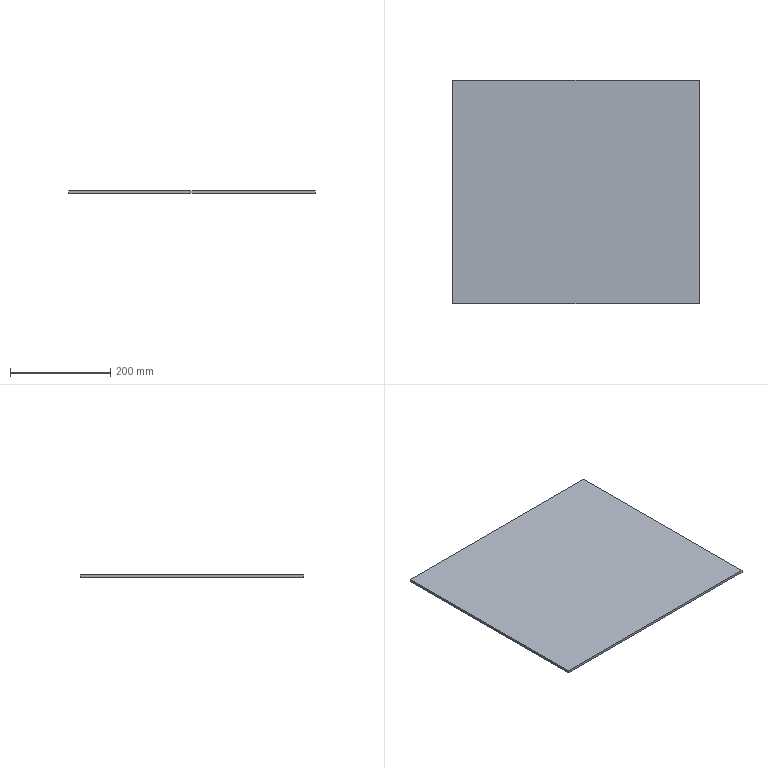Part | NX | features BREP 1 | 1 solid | 6 faces | box 489.9 x 445 x 5 mm | volume 1090028 mm3 | plane 6
STEP:
#1=CARTESIAN_POINT('',(244.95,-222.5,-2.5));
#2=VERTEX_POINT('',#1);
#3=CARTESIAN_POINT('',(244.95,222.5,-2.5));
#4=VERTEX_POINT('',#3);
#5=CARTESIAN_POINT('',(244.95,-222.5,-2.5));
#6=DIRECTION('',(0.,1.,0.));
#7=VECTOR('',#6,1000.);
#8=LINE('',#5,#7);
#9=EDGE_CURVE('',#2,#4,#8,.T.);
#10=ORIENTED_EDGE('',*,*,#9,.T.);
#11=CARTESIAN_POINT('',(244.95,222.5,2.5));
#12=VERTEX_POINT('',#11);
#13=CARTESIAN_POINT('',(244.95,222.5,2.5));
#14=DIRECTION('',(0.,0.,-1.));
#15=VECTOR('',#14,1000.);
#16=LINE('',#13,#15);
#17=EDGE_CURVE('',#12,#4,#16,.T.);
#18=ORIENTED_EDGE('',*,*,#17,.F.);
#19=CARTESIAN_POINT('',(244.95,-222.5,2.5));
#20=VERTEX_POINT('',#19);
#21=CARTESIAN_POINT('',(244.95,-222.5,2.5));
#22=DIRECTION('',(0.,1.,0.));
#23=VECTOR('',#22,1000.);
#24=LINE('',#21,#23);
#25=EDGE_CURVE('',#20,#12,#24,.T.);
#26=ORIENTED_EDGE('',*,*,#25,.F.);
#27=CARTESIAN_POINT('',(244.95,-222.5,2.5));
#28=DIRECTION('',(0.,0.,-1.));
#29=VECTOR('',#28,1000.);
#30=LINE('',#27,#29);
#31=EDGE_CURVE('',#20,#2,#30,.T.);
#32=ORIENTED_EDGE('',*,*,#31,.T.);
#33=EDGE_LOOP('',(#10,#18,#26,#32));
#34=FACE_BOUND('',#33,.T.);
#35=CARTESIAN_POINT('',(244.95,-222.5,2.5));
#36=DIRECTION('',(-1.,0.,0.));
#37=DIRECTION('',(0.,0.,1.));
#38=AXIS2_PLACEMENT_3D('',#35,#36,#37);
#39=PLANE('',#38);
#40=ADVANCED_FACE('',(#34),#39,.F.);
#41=CARTESIAN_POINT('',(-244.95,222.5,-2.5));
#42=VERTEX_POINT('',#41);
#43=CARTESIAN_POINT('',(-244.95,222.5,-2.5));
#44=DIRECTION('',(-1.,0.,0.));
#45=VECTOR('',#44,1000.);
#46=LINE('',#43,#45);
#47=EDGE_CURVE('',#4,#42,#46,.T.);
#48=ORIENTED_EDGE('',*,*,#47,.T.);
#49=CARTESIAN_POINT('',(-244.95,222.5,2.5));
#50=VERTEX_POINT('',#49);
#51=CARTESIAN_POINT('',(-244.95,222.5,2.5));
#52=DIRECTION('',(0.,0.,-1.));
#53=VECTOR('',#52,1000.);
#54=LINE('',#51,#53);
#55=EDGE_CURVE('',#50,#42,#54,.T.);
#56=ORIENTED_EDGE('',*,*,#55,.F.);
#57=CARTESIAN_POINT('',(-244.95,222.5,2.5));
#58=DIRECTION('',(-1.,0.,0.));
#59=VECTOR('',#58,1000.);
#60=LINE('',#57,#59);
#61=EDGE_CURVE('',#12,#50,#60,.T.);
#62=ORIENTED_EDGE('',*,*,#61,.F.);
#63=ORIENTED_EDGE('',*,*,#17,.T.);
#64=EDGE_LOOP('',(#48,#56,#62,#63));
#65=FACE_BOUND('',#64,.T.);
#66=CARTESIAN_POINT('',(-244.95,222.5,2.5));
#67=DIRECTION('',(0.,-1.,0.));
#68=DIRECTION('',(0.,0.,-1.));
#69=AXIS2_PLACEMENT_3D('',#66,#67,#68);
#70=PLANE('',#69);
#71=ADVANCED_FACE('',(#65),#70,.F.);
#72=CARTESIAN_POINT('',(-244.95,-222.5,-2.5));
#73=VERTEX_POINT('',#72);
#74=CARTESIAN_POINT('',(-244.95,-222.5,-2.5));
#75=DIRECTION('',(0.,-1.,0.));
#76=VECTOR('',#75,1000.);
#77=LINE('',#74,#76);
#78=EDGE_CURVE('',#42,#73,#77,.T.);
#79=ORIENTED_EDGE('',*,*,#78,.T.);
#80=CARTESIAN_POINT('',(-244.95,-222.5,2.5));
#81=VERTEX_POINT('',#80);
#82=CARTESIAN_POINT('',(-244.95,-222.5,2.5));
#83=DIRECTION('',(0.,0.,-1.));
#84=VECTOR('',#83,1000.);
#85=LINE('',#82,#84);
#86=EDGE_CURVE('',#81,#73,#85,.T.);
#87=ORIENTED_EDGE('',*,*,#86,.F.);
#88=CARTESIAN_POINT('',(-244.95,-222.5,2.5));
#89=DIRECTION('',(0.,-1.,0.));
#90=VECTOR('',#89,1000.);
#91=LINE('',#88,#90);
#92=EDGE_CURVE('',#50,#81,#91,.T.);
#93=ORIENTED_EDGE('',*,*,#92,.F.);
#94=ORIENTED_EDGE('',*,*,#55,.T.);
#95=EDGE_LOOP('',(#79,#87,#93,#94));
#96=FACE_BOUND('',#95,.T.);
#97=CARTESIAN_POINT('',(-244.95,-222.5,2.5));
#98=DIRECTION('',(1.,0.,0.));
#99=DIRECTION('',(0.,1.,0.));
#100=AXIS2_PLACEMENT_3D('',#97,#98,#99);
#101=PLANE('',#100);
#102=ADVANCED_FACE('',(#96),#101,.F.);
#103=CARTESIAN_POINT('',(-244.95,-222.5,-2.5));
#104=DIRECTION('',(1.,0.,0.));
#105=VECTOR('',#104,1000.);
#106=LINE('',#103,#105);
#107=EDGE_CURVE('',#73,#2,#106,.T.);
#108=ORIENTED_EDGE('',*,*,#107,.T.);
#109=ORIENTED_EDGE('',*,*,#31,.F.);
#110=CARTESIAN_POINT('',(-244.95,-222.5,2.5));
#111=DIRECTION('',(1.,0.,0.));
#112=VECTOR('',#111,1000.);
#113=LINE('',#110,#112);
#114=EDGE_CURVE('',#81,#20,#113,.T.);
#115=ORIENTED_EDGE('',*,*,#114,.F.);
#116=ORIENTED_EDGE('',*,*,#86,.T.);
#117=EDGE_LOOP('',(#108,#109,#115,#116));
#118=FACE_BOUND('',#117,.T.);
#119=CARTESIAN_POINT('',(-244.95,-222.5,2.5));
#120=DIRECTION('',(0.,1.,0.));
#121=DIRECTION('',(1.,0.,0.));
#122=AXIS2_PLACEMENT_3D('',#119,#120,#121);
#123=PLANE('',#122);
#124=ADVANCED_FACE('',(#118),#123,.F.);
#125=ORIENTED_EDGE('',*,*,#25,.T.);
#126=ORIENTED_EDGE('',*,*,#61,.T.);
#127=ORIENTED_EDGE('',*,*,#92,.T.);
#128=ORIENTED_EDGE('',*,*,#114,.T.);
#129=EDGE_LOOP('',(#125,#126,#127,#128));
#130=FACE_BOUND('',#129,.T.);
#131=CARTESIAN_POINT('',(0.,0.,2.5));
#132=DIRECTION('',(0.,0.,-1.));
#133=DIRECTION('',(0.,-1.,0.));
#134=AXIS2_PLACEMENT_3D('',#131,#132,#133);
#135=PLANE('',#134);
#136=ADVANCED_FACE('',(#130),#135,.F.);
#137=ORIENTED_EDGE('',*,*,#9,.F.);
#138=ORIENTED_EDGE('',*,*,#107,.F.);
#139=ORIENTED_EDGE('',*,*,#78,.F.);
#140=ORIENTED_EDGE('',*,*,#47,.F.);
#141=EDGE_LOOP('',(#137,#138,#139,#140));
#142=FACE_BOUND('',#141,.T.);
#143=CARTESIAN_POINT('',(0.,0.,-2.5));
#144=DIRECTION('',(0.,0.,-1.));
#145=DIRECTION('',(0.,-1.,0.));
#146=AXIS2_PLACEMENT_3D('',#143,#144,#145);
#147=PLANE('',#146);
#148=ADVANCED_FACE('',(#142),#147,.T.);
#149=CLOSED_SHELL('',(#40,#71,#102,#124,#136,#148));
#150=MANIFOLD_SOLID_BREP('',#149);
#151=(LENGTH_UNIT()NAMED_UNIT(*)SI_UNIT(.MILLI.,.METRE.));
#152=UNCERTAINTY_MEASURE_WITH_UNIT(LENGTH_MEASURE(0.00001),#151,'','');
#153=(NAMED_UNIT(*)PLANE_ANGLE_UNIT()SI_UNIT($,.RADIAN.));
#154=(NAMED_UNIT(*)SI_UNIT($,.STERADIAN.)SOLID_ANGLE_UNIT());
#155=(GEOMETRIC_REPRESENTATION_CONTEXT(3)GLOBAL_UNCERTAINTY_ASSIGNED_CONTEXT((#152))GLOBAL_UNIT_ASSIGNED_CONTEXT((#151,#153,#154))REPRESENTATION_CONTEXT('',''));
#156=ADVANCED_BREP_SHAPE_REPRESENTATION('',(#150),#155);